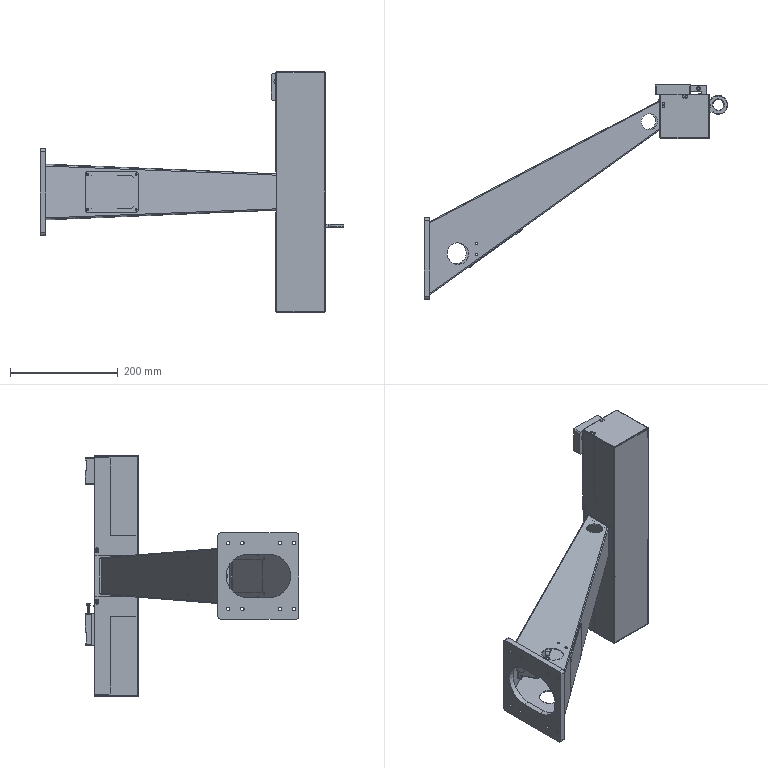Part | SolidWorks | 100 solids | 1733 faces | box 562.593 x 396.277 x 446 mm | volume 1438973 mm3 | plane 733 | cylinder 635 | spline 187 | torus 102 | cone 60 | sphere 16 | commonest cylinder face diameters 4 x63 3.3 x60 4.5 x60 5 x55 3.6 x47 3 x44